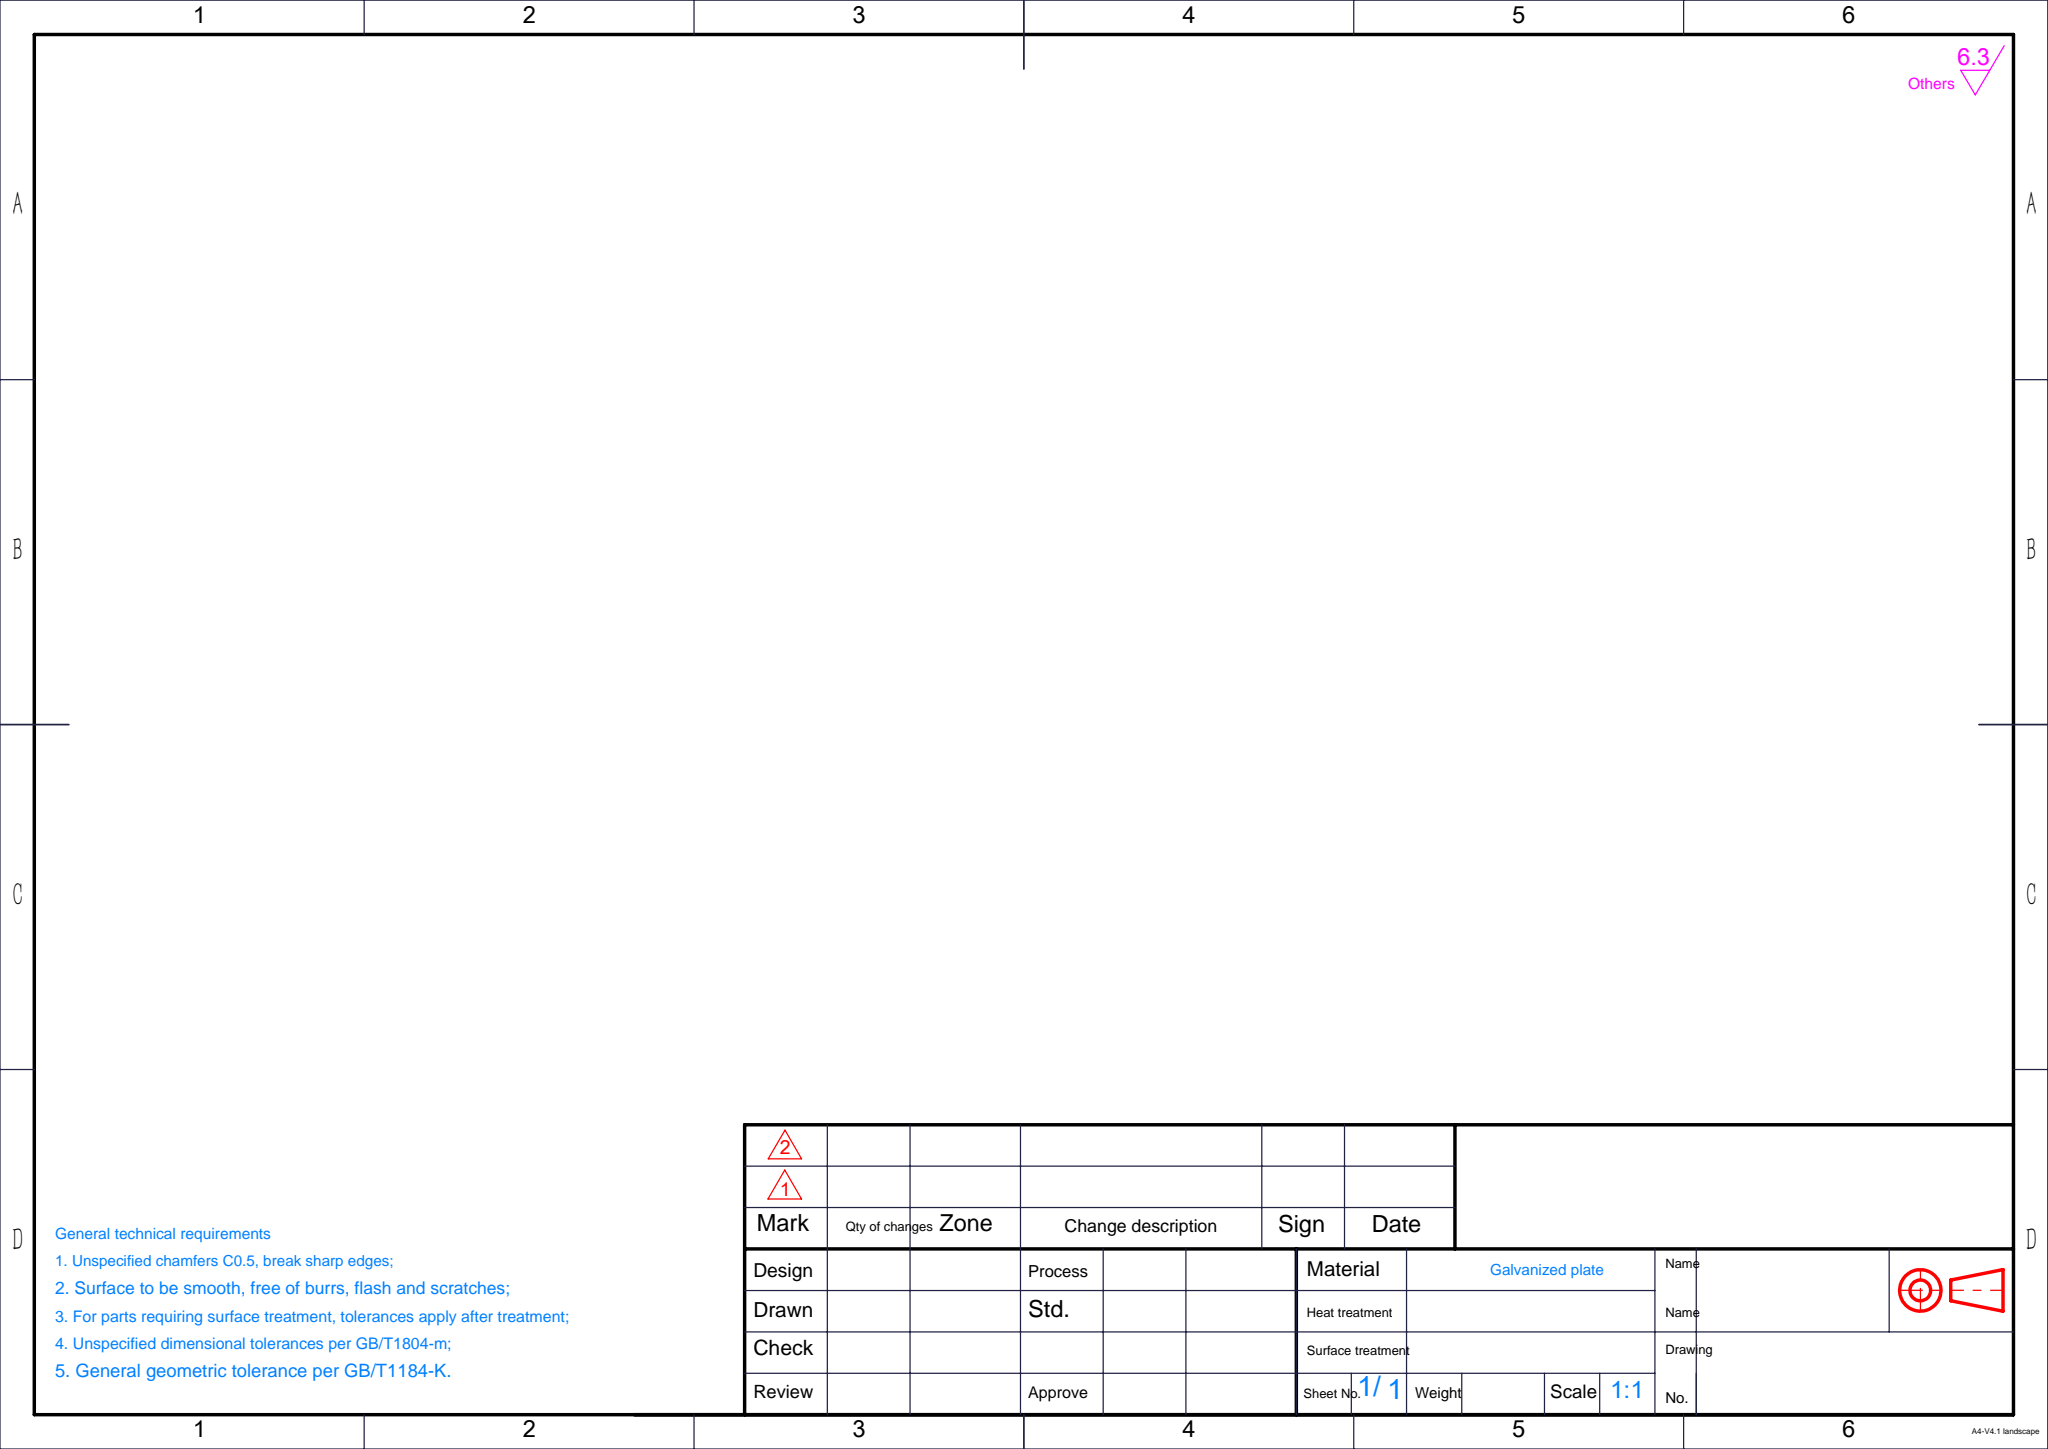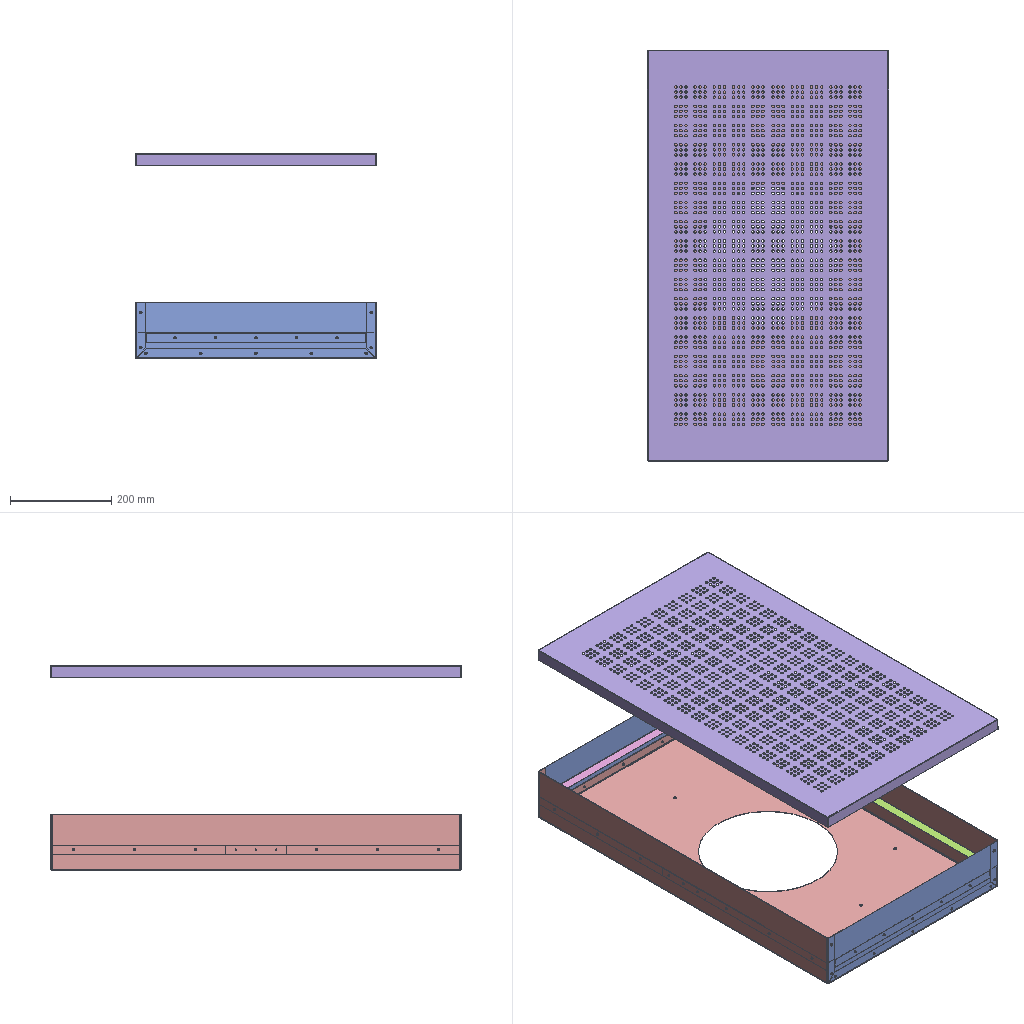Assembly | SolidWorks | 14 different items | 18 placed | box 478 x 814 x 405 mm
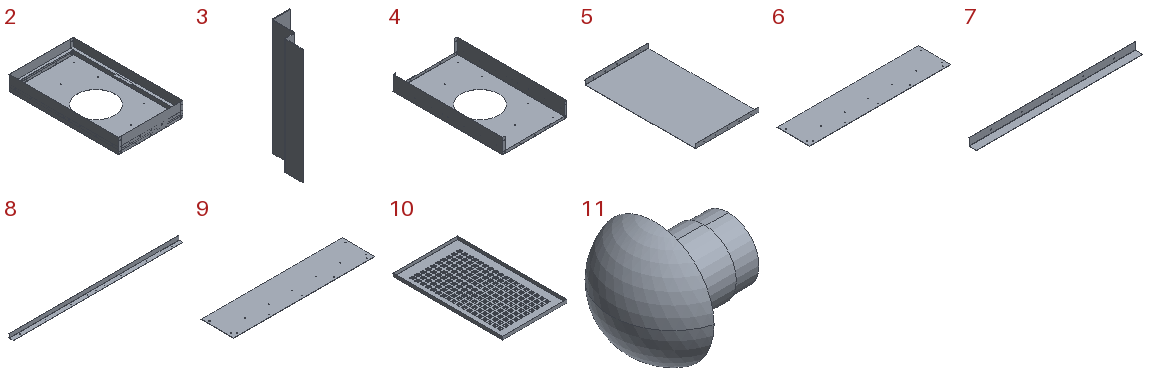Parts list (item | name | quantity | parent item | size | volume | features):
1 | 120 deg blind rivets gb | x1 | - | - | - | -
2 | (subassembly) | x1 | - | 477.6 x 813.6 x 111 mm | 709614 mm3 | features ReferencePattern 23, CompositeCurve 6, MirrorCompFeat 2
3 | - | x2 | in 2 | 30 x 43.6 x 120 mm | 5997 mm3 | features 3DProfileFeature 2, HoleWzd 2, FlatPattern 1, SMBaseFlange 1, SheetMetal 1
4 | - | x1 | in 2 | 475 x 808 x 111 mm | 524962 mm3 | features 3DProfileFeature 5, HoleWzd 5, SketchPattern 4, Chamfer 3, EdgeFlange 2, ICE 2, FlatPattern 1, SMBaseFlange 1, SheetMetal 1
5 | - | x1 | - | 270 x 473 x 20 mm | 137635 mm3 | features 3DProfileFeature 1, EdgeFlange 1, Fillet 1, FlatPattern 1, HoleWzd 1, LPattern 1, MirrorPattern 1, SMBaseFlange 1, SheetMetal 1
6 | - | x1 | - | 473 x 110 x 1 mm | 51967 mm3 | features 3DProfileFeature 1, Chamfer 1, FlatPattern 1, HoleWzd 1, SMBaseFlange 1, SheetMetal 1, SketchPattern 1
7 | - | x2 | in 2 | 433 x 20 x 20 mm | 11755 mm3 | features 3DProfileFeature 1, EdgeFlange 1, FlatPattern 1, HoleWzd 1, LPattern 1, MirrorPattern 1, SMBaseFlange 1, SheetMetal 1
8 | - | x2 | in 2 | 806 x 20 x 20 mm | 21881 mm3 | features 3DProfileFeature 3, HoleWzd 3, EdgeFlange 1, FlatPattern 1, ICE 1, LPattern 1, MirrorPattern 1, SMBaseFlange 1, SheetMetal 1
9 | - | x2 | in 2 | 473 x 110 x 1 mm | 51954 mm3 | features 3DProfileFeature 1, Chamfer 1, FlatPattern 1, HoleWzd 1, ICE 1, SMBaseFlange 1, SheetMetal 1, SketchPattern 1
10 | - | x1 | - | - | 268655 mm3 | features 3DProfileFeature 3, HoleWzd 3, LPattern 3, MirrorPattern 3, EdgeFlange 1, FlatPattern 1, SMBaseFlange 1, SheetMetal 1
11 | - | x1 | - | 4.8 x 4.84 x 4.84 mm | 35.188 mm3 | features Boss 1, RevCut 1, Revolution 1
12 | countersunk head drive rivets gb | x1 | - | - | - | -
13 | rivets for name plate gb | x1 | - | - | - | -
14 | round head rivets gb | x1 | - | - | - | -
Mates (type | each side: item.copy, entity, surface, feature):
In the top assembly
Coincident | 4.1 plane | assembly plane | 3 times
Parallel | 4.1 face plane Base-Flange 1 | 10.1 face plane Base-Flange 1
Parallel | 4.1 face plane Edge-Flange 1 | 10.1 face plane Edge-Flange 1
Coincident | 4.1 face plane Edge-Flange 1 | 10.1 face plane Edge-Flange 1
Coincident | assembly plane | assembly plane | 2 times
Coincident | 8.1 plane | assembly plane
Coincident | 7.1 plane | assembly plane
In subassembly 2
Coincident | 4.2 face plane Edge-Flange 1 | 8.2 face plane Base-Flange 1
DistanceDim | 8.2 face plane Edge-Flange 1 | 4.2 face plane Edge-Flange 1
Coincident | 8.2 face plane Edge-Flange 1 | 7.2 face plane Base-Flange 1
Coincident | 8.2 face plane Edge-Flange 1 | 3.1 face plane Base-Flange 1
Coincident | 8.2 face plane Base-Flange 1 | 3.1 face plane Base-Flange 1
Coincident | 9.1 plane | 2.1 plane
Coincident | 4.2 face plane Edge-Flange 2 | 9.1 face plane Base-Flange 1 | 2 times
Coincident | 7.2 plane | 2.1 plane
Coincident | 8.2 plane | 2.1 plane
Coincident | 3.1 plane | 2.1 plane
Coincident | 9.1 face plane Base-Flange 1 | 7.2 face plane Edge-Flange 1
Concentric | 4.2 edge | 9.2 edge | 2 times
Coincident | 4.2 face plane Edge-Flange 2 | 9.2 face plane Base-Flange 1